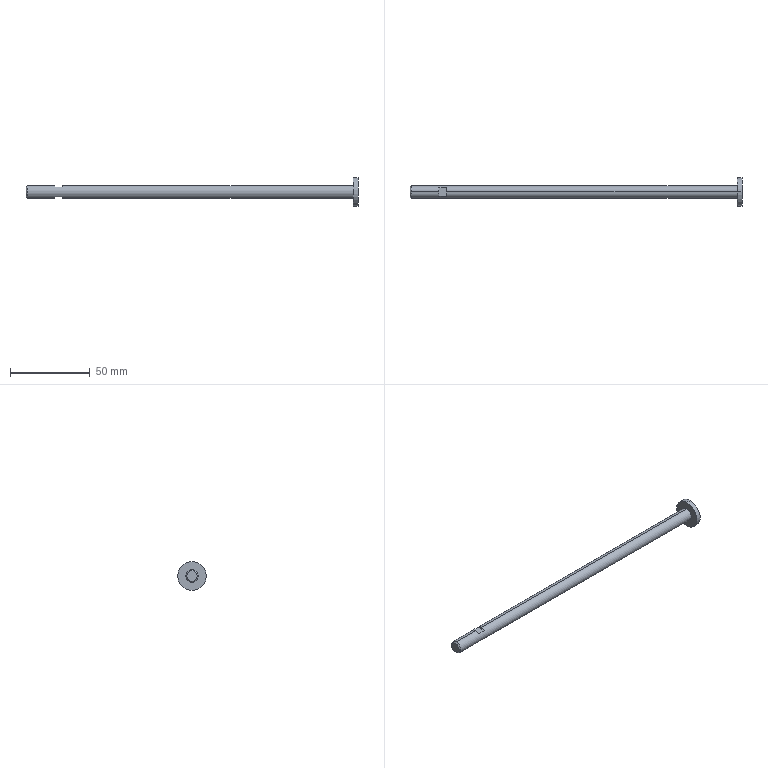Part | SolidWorks | CDM2BZ20x120-D(5)_5.stp | 1 solid | 15 faces | box 208 x 18 x 18 mm | volume 11025 mm3 | plane 9 | cylinder 4 | cone 2 | commonest cylinder face diameters 8 x2 18 x2
STEP:
#1=CARTESIAN_POINT('',(205.,0.,-9.));
#2=VERTEX_POINT('',#1);
#3=CARTESIAN_POINT('',(205.,0.,9.));
#4=VERTEX_POINT('',#3);
#5=CARTESIAN_POINT('',(205.,0.,0.));
#6=DIRECTION('',(1.,0.,0.));
#7=DIRECTION('',(0.,0.,-1.));
#8=AXIS2_PLACEMENT_3D('',#5,#6,#7);
#9=CIRCLE('',#8,9.);
#10=EDGE_CURVE('',#2,#4,#9,.T.);
#11=ORIENTED_EDGE('',*,*,#10,.T.);
#12=CARTESIAN_POINT('',(208.,0.,9.));
#13=VERTEX_POINT('',#12);
#14=CARTESIAN_POINT('',(208.,0.,9.));
#15=DIRECTION('',(1.,0.,0.));
#16=VECTOR('',#15,1000.);
#17=LINE('',#14,#16);
#18=EDGE_CURVE('',#4,#13,#17,.T.);
#19=ORIENTED_EDGE('',*,*,#18,.T.);
#20=CARTESIAN_POINT('',(208.,0.,-9.));
#21=VERTEX_POINT('',#20);
#22=CARTESIAN_POINT('',(208.,0.,0.));
#23=DIRECTION('',(1.,0.,0.));
#24=DIRECTION('',(0.,0.,-1.));
#25=AXIS2_PLACEMENT_3D('',#22,#23,#24);
#26=CIRCLE('',#25,9.);
#27=EDGE_CURVE('',#21,#13,#26,.T.);
#28=ORIENTED_EDGE('',*,*,#27,.F.);
#29=CARTESIAN_POINT('',(208.,0.,-9.));
#30=DIRECTION('',(1.,0.,0.));
#31=VECTOR('',#30,1000.);
#32=LINE('',#29,#31);
#33=EDGE_CURVE('',#2,#21,#32,.T.);
#34=ORIENTED_EDGE('',*,*,#33,.F.);
#35=EDGE_LOOP('',(#11,#19,#28,#34));
#36=FACE_OUTER_BOUND('',#35,.T.);
#37=CARTESIAN_POINT('',(208.,0.,0.));
#38=DIRECTION('',(1.,0.,0.));
#39=DIRECTION('',(0.,0.,-1.));
#40=AXIS2_PLACEMENT_3D('',#37,#38,#39);
#41=CYLINDRICAL_SURFACE('',#40,9.);
#42=ADVANCED_FACE('',(#36),#41,.T.);
#43=CARTESIAN_POINT('',(0.767,0.,-4.));
#44=VERTEX_POINT('',#43);
#45=CARTESIAN_POINT('',(0.767,0.,4.));
#46=VERTEX_POINT('',#45);
#47=CARTESIAN_POINT('',(0.767,0.,0.));
#48=DIRECTION('',(1.,0.,0.));
#49=DIRECTION('',(0.,0.,-1.));
#50=AXIS2_PLACEMENT_3D('',#47,#48,#49);
#51=CIRCLE('',#50,4.);
#52=EDGE_CURVE('',#44,#46,#51,.T.);
#53=ORIENTED_EDGE('',*,*,#52,.T.);
#54=CARTESIAN_POINT('',(18.,0.,4.));
#55=VERTEX_POINT('',#54);
#56=CARTESIAN_POINT('',(208.,0.,4.));
#57=DIRECTION('',(1.,0.,0.));
#58=VECTOR('',#57,1000.);
#59=LINE('',#56,#58);
#60=EDGE_CURVE('',#46,#55,#59,.T.);
#61=ORIENTED_EDGE('',*,*,#60,.T.);
#62=CARTESIAN_POINT('',(18.,2.646,3.));
#63=VERTEX_POINT('',#62);
#64=CARTESIAN_POINT('',(18.,0.,0.));
#65=DIRECTION('',(1.,0.,0.));
#66=DIRECTION('',(0.,0.,-1.));
#67=AXIS2_PLACEMENT_3D('',#64,#65,#66);
#68=CIRCLE('',#67,4.);
#69=EDGE_CURVE('',#63,#55,#68,.T.);
#70=ORIENTED_EDGE('',*,*,#69,.F.);
#71=CARTESIAN_POINT('',(23.,2.646,3.));
#72=VERTEX_POINT('',#71);
#73=CARTESIAN_POINT('',(208.,2.646,3.));
#74=DIRECTION('',(1.,0.,0.));
#75=VECTOR('',#74,1000.);
#76=LINE('',#73,#75);
#77=EDGE_CURVE('',#63,#72,#76,.T.);
#78=ORIENTED_EDGE('',*,*,#77,.T.);
#79=CARTESIAN_POINT('',(23.,0.,4.));
#80=VERTEX_POINT('',#79);
#81=CARTESIAN_POINT('',(23.,0.,0.));
#82=DIRECTION('',(1.,0.,0.));
#83=DIRECTION('',(0.,0.,-1.));
#84=AXIS2_PLACEMENT_3D('',#81,#82,#83);
#85=CIRCLE('',#84,4.);
#86=EDGE_CURVE('',#72,#80,#85,.T.);
#87=ORIENTED_EDGE('',*,*,#86,.T.);
#88=CARTESIAN_POINT('',(205.,0.,4.));
#89=VERTEX_POINT('',#88);
#90=CARTESIAN_POINT('',(208.,0.,4.));
#91=DIRECTION('',(1.,0.,0.));
#92=VECTOR('',#91,1000.);
#93=LINE('',#90,#92);
#94=EDGE_CURVE('',#80,#89,#93,.T.);
#95=ORIENTED_EDGE('',*,*,#94,.T.);
#96=CARTESIAN_POINT('',(205.,0.,-4.));
#97=VERTEX_POINT('',#96);
#98=CARTESIAN_POINT('',(205.,0.,0.));
#99=DIRECTION('',(1.,0.,0.));
#100=DIRECTION('',(0.,0.,-1.));
#101=AXIS2_PLACEMENT_3D('',#98,#99,#100);
#102=CIRCLE('',#101,4.);
#103=EDGE_CURVE('',#97,#89,#102,.T.);
#104=ORIENTED_EDGE('',*,*,#103,.F.);
#105=CARTESIAN_POINT('',(23.,0.,-4.));
#106=VERTEX_POINT('',#105);
#107=CARTESIAN_POINT('',(208.,0.,-4.));
#108=DIRECTION('',(1.,0.,0.));
#109=VECTOR('',#108,1000.);
#110=LINE('',#107,#109);
#111=EDGE_CURVE('',#106,#97,#110,.T.);
#112=ORIENTED_EDGE('',*,*,#111,.F.);
#113=CARTESIAN_POINT('',(23.,2.646,-3.));
#114=VERTEX_POINT('',#113);
#115=CARTESIAN_POINT('',(23.,0.,0.));
#116=DIRECTION('',(1.,0.,0.));
#117=DIRECTION('',(0.,0.,-1.));
#118=AXIS2_PLACEMENT_3D('',#115,#116,#117);
#119=CIRCLE('',#118,4.);
#120=EDGE_CURVE('',#106,#114,#119,.T.);
#121=ORIENTED_EDGE('',*,*,#120,.T.);
#122=CARTESIAN_POINT('',(18.,2.646,-3.));
#123=VERTEX_POINT('',#122);
#124=CARTESIAN_POINT('',(208.,2.646,-3.));
#125=DIRECTION('',(-1.,0.,0.));
#126=VECTOR('',#125,1000.);
#127=LINE('',#124,#126);
#128=EDGE_CURVE('',#114,#123,#127,.T.);
#129=ORIENTED_EDGE('',*,*,#128,.T.);
#130=CARTESIAN_POINT('',(18.,0.,-4.));
#131=VERTEX_POINT('',#130);
#132=CARTESIAN_POINT('',(18.,0.,0.));
#133=DIRECTION('',(1.,0.,0.));
#134=DIRECTION('',(0.,0.,-1.));
#135=AXIS2_PLACEMENT_3D('',#132,#133,#134);
#136=CIRCLE('',#135,4.);
#137=EDGE_CURVE('',#131,#123,#136,.T.);
#138=ORIENTED_EDGE('',*,*,#137,.F.);
#139=CARTESIAN_POINT('',(208.,0.,-4.));
#140=DIRECTION('',(1.,0.,0.));
#141=VECTOR('',#140,1000.);
#142=LINE('',#139,#141);
#143=EDGE_CURVE('',#44,#131,#142,.T.);
#144=ORIENTED_EDGE('',*,*,#143,.F.);
#145=EDGE_LOOP('',(#53,#61,#70,#78,#87,#95,#104,#112,#121,#129,#138,#144));
#146=FACE_OUTER_BOUND('',#145,.T.);
#147=CARTESIAN_POINT('',(208.,0.,0.));
#148=DIRECTION('',(1.,0.,0.));
#149=DIRECTION('',(0.,0.,-1.));
#150=AXIS2_PLACEMENT_3D('',#147,#148,#149);
#151=CYLINDRICAL_SURFACE('',#150,4.);
#152=ADVANCED_FACE('',(#146),#151,.T.);
#153=CARTESIAN_POINT('',(0.,0.,-3.233));
#154=VERTEX_POINT('',#153);
#155=CARTESIAN_POINT('',(0.,0.,3.233));
#156=VERTEX_POINT('',#155);
#157=CARTESIAN_POINT('',(0.,0.,0.));
#158=DIRECTION('',(1.,0.,0.));
#159=DIRECTION('',(0.,0.,-1.));
#160=AXIS2_PLACEMENT_3D('',#157,#158,#159);
#161=CIRCLE('',#160,3.233);
#162=EDGE_CURVE('',#154,#156,#161,.T.);
#163=ORIENTED_EDGE('',*,*,#162,.T.);
#164=CARTESIAN_POINT('',(0.,0.,3.233));
#165=DIRECTION('',(0.7071,0.,0.7071));
#166=VECTOR('',#165,1000.);
#167=LINE('',#164,#166);
#168=EDGE_CURVE('',#156,#46,#167,.T.);
#169=ORIENTED_EDGE('',*,*,#168,.T.);
#170=ORIENTED_EDGE('',*,*,#52,.F.);
#171=CARTESIAN_POINT('',(0.,0.,-3.233));
#172=DIRECTION('',(0.7071,0.,-0.7071));
#173=VECTOR('',#172,1000.);
#174=LINE('',#171,#173);
#175=EDGE_CURVE('',#154,#44,#174,.T.);
#176=ORIENTED_EDGE('',*,*,#175,.F.);
#177=EDGE_LOOP('',(#163,#169,#170,#176));
#178=FACE_OUTER_BOUND('',#177,.T.);
#179=CARTESIAN_POINT('',(0.,0.,0.));
#180=DIRECTION('',(1.,0.,0.));
#181=DIRECTION('',(0.,0.,-1.));
#182=AXIS2_PLACEMENT_3D('',#179,#180,#181);
#183=CONICAL_SURFACE('',#182,3.233,0.7854);
#184=ADVANCED_FACE('',(#178),#183,.T.);
#185=ORIENTED_EDGE('',*,*,#162,.F.);
#186=CARTESIAN_POINT('',(0.,0.,0.));
#187=DIRECTION('',(1.,0.,0.));
#188=DIRECTION('',(0.,0.,-1.));
#189=AXIS2_PLACEMENT_3D('',#186,#187,#188);
#190=CIRCLE('',#189,3.233);
#191=EDGE_CURVE('',#156,#154,#190,.T.);
#192=ORIENTED_EDGE('',*,*,#191,.F.);
#193=EDGE_LOOP('',(#185,#192));
#194=FACE_OUTER_BOUND('',#193,.T.);
#195=CARTESIAN_POINT('',(0.,0.,0.));
#196=DIRECTION('',(1.,0.,0.));
#197=DIRECTION('',(0.,1.,0.));
#198=AXIS2_PLACEMENT_3D('',#195,#196,#197);
#199=PLANE('',#198);
#200=ADVANCED_FACE('',(#194),#199,.F.);
#201=ORIENTED_EDGE('',*,*,#168,.F.);
#202=ORIENTED_EDGE('',*,*,#191,.T.);
#203=ORIENTED_EDGE('',*,*,#175,.T.);
#204=CARTESIAN_POINT('',(0.767,0.,0.));
#205=DIRECTION('',(1.,0.,0.));
#206=DIRECTION('',(0.,0.,-1.));
#207=AXIS2_PLACEMENT_3D('',#204,#205,#206);
#208=CIRCLE('',#207,4.);
#209=EDGE_CURVE('',#46,#44,#208,.T.);
#210=ORIENTED_EDGE('',*,*,#209,.F.);
#211=EDGE_LOOP('',(#201,#202,#203,#210));
#212=FACE_OUTER_BOUND('',#211,.T.);
#213=CARTESIAN_POINT('',(0.,0.,0.));
#214=DIRECTION('',(1.,0.,0.));
#215=DIRECTION('',(0.,0.,-1.));
#216=AXIS2_PLACEMENT_3D('',#213,#214,#215);
#217=CONICAL_SURFACE('',#216,3.233,0.7854);
#218=ADVANCED_FACE('',(#212),#217,.T.);
#219=ORIENTED_EDGE('',*,*,#60,.F.);
#220=ORIENTED_EDGE('',*,*,#209,.T.);
#221=ORIENTED_EDGE('',*,*,#143,.T.);
#222=CARTESIAN_POINT('',(18.,-2.646,-3.));
#223=VERTEX_POINT('',#222);
#224=CARTESIAN_POINT('',(18.,0.,0.));
#225=DIRECTION('',(1.,0.,0.));
#226=DIRECTION('',(0.,0.,-1.));
#227=AXIS2_PLACEMENT_3D('',#224,#225,#226);
#228=CIRCLE('',#227,4.);
#229=EDGE_CURVE('',#223,#131,#228,.T.);
#230=ORIENTED_EDGE('',*,*,#229,.F.);
#231=CARTESIAN_POINT('',(23.,-2.646,-3.));
#232=VERTEX_POINT('',#231);
#233=CARTESIAN_POINT('',(208.,-2.646,-3.));
#234=DIRECTION('',(1.,0.,0.));
#235=VECTOR('',#234,1000.);
#236=LINE('',#233,#235);
#237=EDGE_CURVE('',#223,#232,#236,.T.);
#238=ORIENTED_EDGE('',*,*,#237,.T.);
#239=CARTESIAN_POINT('',(23.,0.,0.));
#240=DIRECTION('',(1.,0.,0.));
#241=DIRECTION('',(0.,0.,-1.));
#242=AXIS2_PLACEMENT_3D('',#239,#240,#241);
#243=CIRCLE('',#242,4.);
#244=EDGE_CURVE('',#232,#106,#243,.T.);
#245=ORIENTED_EDGE('',*,*,#244,.T.);
#246=ORIENTED_EDGE('',*,*,#111,.T.);
#247=CARTESIAN_POINT('',(205.,0.,0.));
#248=DIRECTION('',(1.,0.,0.));
#249=DIRECTION('',(0.,0.,-1.));
#250=AXIS2_PLACEMENT_3D('',#247,#248,#249);
#251=CIRCLE('',#250,4.);
#252=EDGE_CURVE('',#89,#97,#251,.T.);
#253=ORIENTED_EDGE('',*,*,#252,.F.);
#254=ORIENTED_EDGE('',*,*,#94,.F.);
#255=CARTESIAN_POINT('',(23.,-2.646,3.));
#256=VERTEX_POINT('',#255);
#257=CARTESIAN_POINT('',(23.,0.,0.));
#258=DIRECTION('',(1.,0.,0.));
#259=DIRECTION('',(0.,0.,-1.));
#260=AXIS2_PLACEMENT_3D('',#257,#258,#259);
#261=CIRCLE('',#260,4.);
#262=EDGE_CURVE('',#80,#256,#261,.T.);
#263=ORIENTED_EDGE('',*,*,#262,.T.);
#264=CARTESIAN_POINT('',(18.,-2.646,3.));
#265=VERTEX_POINT('',#264);
#266=CARTESIAN_POINT('',(208.,-2.646,3.));
#267=DIRECTION('',(-1.,0.,0.));
#268=VECTOR('',#267,1000.);
#269=LINE('',#266,#268);
#270=EDGE_CURVE('',#256,#265,#269,.T.);
#271=ORIENTED_EDGE('',*,*,#270,.T.);
#272=CARTESIAN_POINT('',(18.,0.,0.));
#273=DIRECTION('',(1.,0.,0.));
#274=DIRECTION('',(0.,0.,-1.));
#275=AXIS2_PLACEMENT_3D('',#272,#273,#274);
#276=CIRCLE('',#275,4.);
#277=EDGE_CURVE('',#55,#265,#276,.T.);
#278=ORIENTED_EDGE('',*,*,#277,.F.);
#279=EDGE_LOOP('',(#219,#220,#221,#230,#238,#245,#246,#253,#254,#263,#271,#278));
#280=FACE_OUTER_BOUND('',#279,.T.);
#281=CARTESIAN_POINT('',(208.,0.,0.));
#282=DIRECTION('',(1.,0.,0.));
#283=DIRECTION('',(0.,0.,-1.));
#284=AXIS2_PLACEMENT_3D('',#281,#282,#283);
#285=CYLINDRICAL_SURFACE('',#284,4.);
#286=ADVANCED_FACE('',(#280),#285,.T.);
#287=ORIENTED_EDGE('',*,*,#10,.F.);
#288=CARTESIAN_POINT('',(205.,0.,0.));
#289=DIRECTION('',(1.,0.,0.));
#290=DIRECTION('',(0.,0.,-1.));
#291=AXIS2_PLACEMENT_3D('',#288,#289,#290);
#292=CIRCLE('',#291,9.);
#293=EDGE_CURVE('',#4,#2,#292,.T.);
#294=ORIENTED_EDGE('',*,*,#293,.F.);
#295=EDGE_LOOP('',(#287,#294));
#296=FACE_OUTER_BOUND('',#295,.T.);
#297=ORIENTED_EDGE('',*,*,#103,.T.);
#298=ORIENTED_EDGE('',*,*,#252,.T.);
#299=EDGE_LOOP('',(#297,#298));
#300=FACE_BOUND('',#299,.T.);
#301=CARTESIAN_POINT('',(205.,4.,0.));
#302=DIRECTION('',(1.,0.,0.));
#303=DIRECTION('',(0.,1.,0.));
#304=AXIS2_PLACEMENT_3D('',#301,#302,#303);
#305=PLANE('',#304);
#306=ADVANCED_FACE('',(#296,#300),#305,.F.);
#307=ORIENTED_EDGE('',*,*,#18,.F.);
#308=ORIENTED_EDGE('',*,*,#293,.T.);
#309=ORIENTED_EDGE('',*,*,#33,.T.);
#310=CARTESIAN_POINT('',(208.,0.,0.));
#311=DIRECTION('',(1.,0.,0.));
#312=DIRECTION('',(0.,0.,-1.));
#313=AXIS2_PLACEMENT_3D('',#310,#311,#312);
#314=CIRCLE('',#313,9.);
#315=EDGE_CURVE('',#13,#21,#314,.T.);
#316=ORIENTED_EDGE('',*,*,#315,.F.);
#317=EDGE_LOOP('',(#307,#308,#309,#316));
#318=FACE_OUTER_BOUND('',#317,.T.);
#319=CARTESIAN_POINT('',(208.,0.,0.));
#320=DIRECTION('',(1.,0.,0.));
#321=DIRECTION('',(0.,0.,-1.));
#322=AXIS2_PLACEMENT_3D('',#319,#320,#321);
#323=CYLINDRICAL_SURFACE('',#322,9.);
#324=ADVANCED_FACE('',(#318),#323,.T.);
#325=ORIENTED_EDGE('',*,*,#27,.T.);
#326=ORIENTED_EDGE('',*,*,#315,.T.);
#327=EDGE_LOOP('',(#325,#326));
#328=FACE_OUTER_BOUND('',#327,.T.);
#329=CARTESIAN_POINT('',(208.,9.,0.));
#330=DIRECTION('',(-1.,0.,0.));
#331=DIRECTION('',(0.,0.,1.));
#332=AXIS2_PLACEMENT_3D('',#329,#330,#331);
#333=PLANE('',#332);
#334=ADVANCED_FACE('',(#328),#333,.F.);
#335=CARTESIAN_POINT('',(23.,-50.,-3.));
#336=DIRECTION('',(0.,1.,0.));
#337=VECTOR('',#336,1000.);
#338=LINE('',#335,#337);
#339=EDGE_CURVE('',#232,#114,#338,.T.);
#340=ORIENTED_EDGE('',*,*,#339,.T.);
#341=ORIENTED_EDGE('',*,*,#120,.F.);
#342=ORIENTED_EDGE('',*,*,#244,.F.);
#343=EDGE_LOOP('',(#340,#341,#342));
#344=FACE_OUTER_BOUND('',#343,.T.);
#345=CARTESIAN_POINT('',(23.,0.,0.));
#346=DIRECTION('',(1.,0.,0.));
#347=DIRECTION('',(0.,1.,0.));
#348=AXIS2_PLACEMENT_3D('',#345,#346,#347);
#349=PLANE('',#348);
#350=ADVANCED_FACE('',(#344),#349,.F.);
#351=ORIENTED_EDGE('',*,*,#229,.T.);
#352=ORIENTED_EDGE('',*,*,#137,.T.);
#353=CARTESIAN_POINT('',(18.,-50.,-3.));
#354=DIRECTION('',(0.,1.,0.));
#355=VECTOR('',#354,1000.);
#356=LINE('',#353,#355);
#357=EDGE_CURVE('',#223,#123,#356,.T.);
#358=ORIENTED_EDGE('',*,*,#357,.F.);
#359=EDGE_LOOP('',(#351,#352,#358));
#360=FACE_OUTER_BOUND('',#359,.T.);
#361=CARTESIAN_POINT('',(18.,0.,0.));
#362=DIRECTION('',(1.,0.,0.));
#363=DIRECTION('',(0.,1.,0.));
#364=AXIS2_PLACEMENT_3D('',#361,#362,#363);
#365=PLANE('',#364);
#366=ADVANCED_FACE('',(#360),#365,.T.);
#367=ORIENTED_EDGE('',*,*,#357,.T.);
#368=ORIENTED_EDGE('',*,*,#128,.F.);
#369=ORIENTED_EDGE('',*,*,#339,.F.);
#370=ORIENTED_EDGE('',*,*,#237,.F.);
#371=EDGE_LOOP('',(#367,#368,#369,#370));
#372=FACE_OUTER_BOUND('',#371,.T.);
#373=CARTESIAN_POINT('',(23.,-50.,-3.));
#374=DIRECTION('',(0.,0.,1.));
#375=DIRECTION('',(0.,-1.,0.));
#376=AXIS2_PLACEMENT_3D('',#373,#374,#375);
#377=PLANE('',#376);
#378=ADVANCED_FACE('',(#372),#377,.F.);
#379=CARTESIAN_POINT('',(18.,50.,3.));
#380=DIRECTION('',(0.,-1.,0.));
#381=VECTOR('',#380,1000.);
#382=LINE('',#379,#381);
#383=EDGE_CURVE('',#63,#265,#382,.T.);
#384=ORIENTED_EDGE('',*,*,#383,.T.);
#385=ORIENTED_EDGE('',*,*,#270,.F.);
#386=CARTESIAN_POINT('',(23.,50.,3.));
#387=DIRECTION('',(0.,-1.,0.));
#388=VECTOR('',#387,1000.);
#389=LINE('',#386,#388);
#390=EDGE_CURVE('',#72,#256,#389,.T.);
#391=ORIENTED_EDGE('',*,*,#390,.F.);
#392=ORIENTED_EDGE('',*,*,#77,.F.);
#393=EDGE_LOOP('',(#384,#385,#391,#392));
#394=FACE_OUTER_BOUND('',#393,.T.);
#395=CARTESIAN_POINT('',(23.,50.,3.));
#396=DIRECTION('',(0.,0.,-1.));
#397=DIRECTION('',(-1.,0.,0.));
#398=AXIS2_PLACEMENT_3D('',#395,#396,#397);
#399=PLANE('',#398);
#400=ADVANCED_FACE('',(#394),#399,.F.);
#401=ORIENTED_EDGE('',*,*,#390,.T.);
#402=ORIENTED_EDGE('',*,*,#262,.F.);
#403=ORIENTED_EDGE('',*,*,#86,.F.);
#404=EDGE_LOOP('',(#401,#402,#403));
#405=FACE_OUTER_BOUND('',#404,.T.);
#406=CARTESIAN_POINT('',(23.,0.,0.));
#407=DIRECTION('',(1.,0.,0.));
#408=DIRECTION('',(0.,1.,0.));
#409=AXIS2_PLACEMENT_3D('',#406,#407,#408);
#410=PLANE('',#409);
#411=ADVANCED_FACE('',(#405),#410,.F.);
#412=ORIENTED_EDGE('',*,*,#69,.T.);
#413=ORIENTED_EDGE('',*,*,#277,.T.);
#414=ORIENTED_EDGE('',*,*,#383,.F.);
#415=EDGE_LOOP('',(#412,#413,#414));
#416=FACE_OUTER_BOUND('',#415,.T.);
#417=CARTESIAN_POINT('',(18.,0.,0.));
#418=DIRECTION('',(1.,0.,0.));
#419=DIRECTION('',(0.,1.,0.));
#420=AXIS2_PLACEMENT_3D('',#417,#418,#419);
#421=PLANE('',#420);
#422=ADVANCED_FACE('',(#416),#421,.T.);
#423=CLOSED_SHELL('',(#42,#152,#184,#200,#218,#286,#306,#324,#334,#350,#366,#378,#400,#411,#422));
#424=MANIFOLD_SOLID_BREP('',#423);
#425=CARTESIAN_POINT('',(0.,0.,0.));
#426=DIRECTION('',(0.,0.,1.));
#427=DIRECTION('',(1.,0.,0.));
#428=AXIS2_PLACEMENT_3D('',#425,#426,#427);
#429=(LENGTH_UNIT()NAMED_UNIT(*)SI_UNIT(.MILLI.,.METRE.));
#430=UNCERTAINTY_MEASURE_WITH_UNIT(LENGTH_MEASURE(0.00001),#429,'','');
#431=(NAMED_UNIT(*)PLANE_ANGLE_UNIT()SI_UNIT($,.RADIAN.));
#432=(NAMED_UNIT(*)SI_UNIT($,.STERADIAN.)SOLID_ANGLE_UNIT());
#433=(GEOMETRIC_REPRESENTATION_CONTEXT(3)GLOBAL_UNCERTAINTY_ASSIGNED_CONTEXT((#430))GLOBAL_UNIT_ASSIGNED_CONTEXT((#429,#431,#432))REPRESENTATION_CONTEXT('',''));
#434=ADVANCED_BREP_SHAPE_REPRESENTATION('',(#424,#428),#433);